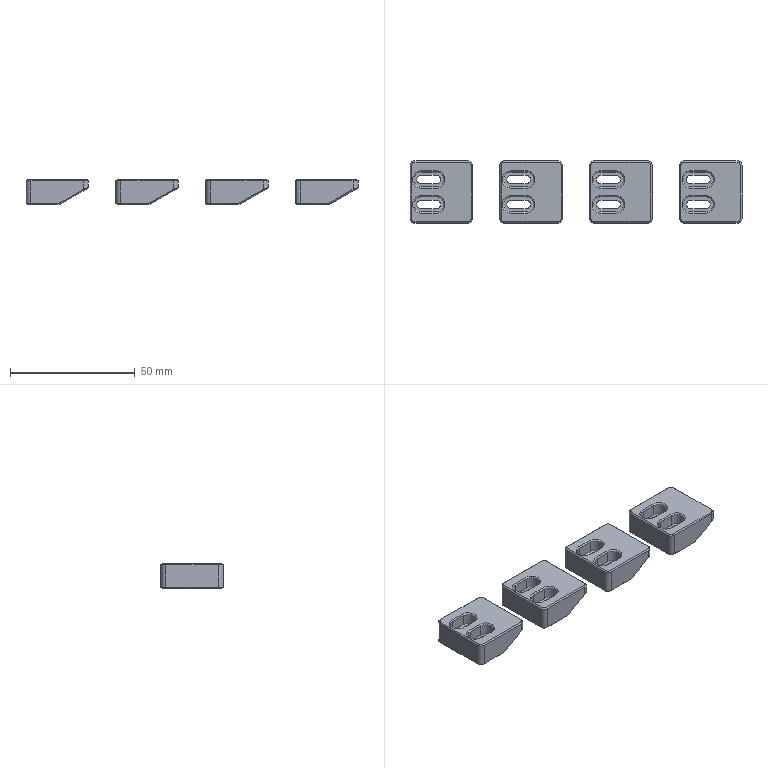NC program | NX | posted with a generic post | part box 133 x 25 x 10 mm
Lines 51 to 970 of 3677:
(ZLEVEL_PROFILE_COPY_COPY , TOOL : D4)
N100 T11 M6
N102 G54
N104 G17 G0 G90 X59.704 Y-4. S9500 M3
N106 G43 Z30. H11
N108 Z1.5
N110 G94 G1 X55.905 Z1.301 F1350.
N112 X55.631 Y-4.061 Z1.286
N114 X55.457 Y-4.158 Z1.276
N116 X55.261 Y-4.358 Z1.261
N118 X55.11 Y-4.603 Z1.246
N120 X55.004 Y-4.807 Z1.234
N122 X55.003 Y-5.188 Z1.214
N124 X55.113 Y-5.404 Z1.201
N126 X55.192 Y-5.615 Z1.19
N128 X55.32 Y-5.757 Z1.179
N130 X55.53 Y-5.86 Z1.167
N132 X55.597 Y-5.888 Z1.163
N134 X55.987 Y-5.982 Z1.142
N136 Y-6. Z1.141
N138 X62.118 Z0.82
N140 X62.329 Y-5.926 Z0.808
N142 X62.561 Y-5.847 Z0.796
N144 X62.879 Y-5.518 Z0.772
N146 X63.02 Y-5.083 Z0.748
N148 X62.944 Y-4.599 Z0.722
N150 X62.674 Y-4.229 Z0.698
N152 X62.269 Y-4.015 Z0.674
N154 X62.025 Y-4.012 Z0.661
N156 Y-4.
N158 X55.905 Z0.34
N160 X55.631 Y-4.061 Z0.325
N162 X55.457 Y-4.158 Z0.315
N164 X55.261 Y-4.358 Z0.3
N166 X55.11 Y-4.603 Z0.285
N168 X55.004 Y-4.807 Z0.273
N170 X55.003 Y-5.188 Z0.253
N172 X55.113 Y-5.404 Z0.24
N174 X55.192 Y-5.615 Z0.228
N176 X55.32 Y-5.757 Z0.218
N178 X55.53 Y-5.86 Z0.206
N180 X55.597 Y-5.888 Z0.202
N182 X55.987 Y-5.982 Z0.181
N184 Y-6. Z0.18
N186 X62.118 Z-0.141
N188 X62.329 Y-5.926 Z-0.153
N190 X62.561 Y-5.847 Z-0.166
N192 X62.879 Y-5.518 Z-0.19
N194 X63.02 Y-5.083 Z-0.214
N196 X62.944 Y-4.599 Z-0.239
N198 X62.674 Y-4.229 Z-0.263
N200 X62.269 Y-4.015 Z-0.287
N202 X62.025 Y-4.012 Z-0.3
N204 Y-4.
N206 X55.905
N208 G3 X55.261 Y-4.358 R1.295
N210 G1 X55.11 Y-4.603
N212 G3 X55.113 Y-5.404 R0.863
N214 X55.53 Y-5.86 R0.828
N216 G1 X55.597 Y-5.888
N218 X55.987 Y-5.982
N220 Y-6.
N222 X62.118
N224 X62.329 Y-5.926
N226 G3 X62.025 Y-4.012 R0.984
N228 G1 X61.786 Y-4. Z-0.305
N230 X61.548 Z-0.311
N232 X56.176 Z-0.429
N234 X55.822 Y-4.041 Z-0.436
N236 X55.7 Y-4.069 Z-0.439
N238 X55.438 Y-4.201 Z-0.446
N240 X55.288 Y-4.326 Z-0.45
N242 X55.128 Y-4.561 Z-0.456
N244 X55.049 Y-4.75 Z-0.461
N246 X55.027 Y-4.927 Z-0.465
N248 X55.019 Y-5.016 Z-0.467
N250 X55.029 Y-5.087 Z-0.468
N252 X55.048 Y-5.231 Z-0.471
N254 X55.114 Y-5.41 Z-0.476
N256 X55.152 Y-5.497 Z-0.478
N258 X55.275 Y-5.656 Z-0.482
N260 X55.407 Y-5.775 Z-0.486
N262 X55.478 Y-5.828 Z-0.488
N264 X55.541 Y-5.864 Z-0.49
N266 X55.677 Y-5.92 Z-0.493
N268 X55.877 Y-5.967 Z-0.498
N270 X56.141 Y-6. Z-0.504
N272 X60.536 Z-0.6
N274 X62.
N276 G3 X62.025 Y-4. R1.
N278 G1 X61.78 Z-0.605
N280 X59.576 Z-0.654
N282 X57.617 Z-0.696
N284 X57.372 Y-4.001 Z-0.702
N286 X57.128 Y-4. Z-0.707
N288 X56.148 Z-0.729
N290 X55.807 Y-4.043 Z-0.736
N292 X55.673 Y-4.08 Z-0.739
N294 X55.42 Y-4.218 Z-0.746
N296 X55.277 Y-4.34 Z-0.75
N298 X55.123 Y-4.571 Z-0.756
N300 X55.048 Y-4.757 Z-0.761
N302 X55.02 Y-5.023 Z-0.767
N304 X55.048 Y-5.233 Z-0.771
N306 X55.112 Y-5.406 Z-0.776
N308 X55.149 Y-5.491 Z-0.778
N310 X55.271 Y-5.652 Z-0.782
N312 X55.404 Y-5.771 Z-0.786
N314 X55.474 Y-5.826 Z-0.788
N316 X55.533 Y-5.862 Z-0.79
N318 X55.664 Y-5.917 Z-0.793
N320 X55.868 Y-5.965 Z-0.798
N322 X56.138 Y-6. Z-0.804
N324 X60.546 Z-0.9
N326 X62.
N328 G3 X62.025 Y-4. R1.
N330 G1 X61.78 Z-0.905
N332 X59.576 Z-0.954
N334 X56.638 Z-1.018
N336 X56.393 Y-4.001 Z-1.023
N338 X56.148 Y-4. Z-1.029
N340 X55.809 Y-4.043 Z-1.036
N342 X55.673 Y-4.08 Z-1.039
N344 X55.421 Y-4.217 Z-1.046
N346 X55.277 Y-4.341 Z-1.05
N348 X55.123 Y-4.571 Z-1.056
N350 X55.048 Y-4.757 Z-1.061
N352 X55.021 Y-5.023 Z-1.067
N354 X55.048 Y-5.233 Z-1.071
N356 X55.113 Y-5.406 Z-1.076
N358 X55.149 Y-5.49 Z-1.078
N360 X55.271 Y-5.652 Z-1.082
N362 X55.404 Y-5.771 Z-1.086
N364 X55.474 Y-5.825 Z-1.088
N366 X55.533 Y-5.862 Z-1.09
N368 X55.664 Y-5.917 Z-1.093
N370 X55.868 Y-5.965 Z-1.098
N372 X56.138 Y-6. Z-1.104
N374 X60.546 Z-1.2
N376 X62.
N378 G3 X62.025 Y-4. R1.
N380 G1 X61.78 Z-1.205
N382 X59.576 Z-1.254
N384 X56.148 Z-1.329
N386 X55.807 Y-4.043 Z-1.336
N388 X55.673 Y-4.08 Z-1.339
N390 X55.419 Y-4.216 Z-1.346
N392 X55.277 Y-4.341 Z-1.35
N394 X55.121 Y-4.575 Z-1.356
N396 X55.048 Y-4.757 Z-1.361
N398 X55.021 Y-5.024 Z-1.367
N400 X55.048 Y-5.233 Z-1.371
N402 X55.113 Y-5.406 Z-1.376
N404 X55.15 Y-5.49 Z-1.378
N406 X55.271 Y-5.652 Z-1.382
N408 X55.404 Y-5.77 Z-1.386
N410 X55.474 Y-5.825 Z-1.388
N412 X55.533 Y-5.862 Z-1.39
N414 X55.664 Y-5.917 Z-1.393
N416 X55.868 Y-5.965 Z-1.398
N418 X56.138 Y-6. Z-1.404
N420 X60.546 Z-1.5
N422 X62.
N424 G3 X62.025 Y-4. R1.
N426 G1 X61.78 Z-1.505
N428 X59.576 Z-1.554
N430 X56.148 Z-1.629
N432 X55.807 Y-4.043 Z-1.636
N434 X55.673 Y-4.08 Z-1.639
N436 X55.42 Y-4.216 Z-1.646
N438 X55.277 Y-4.341 Z-1.65
N440 X55.122 Y-4.575 Z-1.656
N442 X55.048 Y-4.757 Z-1.661
N444 X55.021 Y-5.023 Z-1.667
N446 X55.048 Y-5.233 Z-1.671
N448 X55.113 Y-5.406 Z-1.676
N450 X55.15 Y-5.49 Z-1.678
N452 X55.271 Y-5.652 Z-1.682
N454 X55.404 Y-5.77 Z-1.686
N456 X55.473 Y-5.824 Z-1.688
N458 X55.533 Y-5.861 Z-1.69
N460 X55.664 Y-5.917 Z-1.693
N462 X55.867 Y-5.964 Z-1.698
N464 X56.138 Y-6. Z-1.704
N466 X60.546 Z-1.8
N468 X62.
N470 G3 X62.025 Y-4. R1.
N472 G1 X61.78 Z-1.805
N474 X59.576 Z-1.854
N476 X57.128 Z-1.907
N478 X56.883 Y-4.001 Z-1.913
N480 X56.638 Y-4. Z-1.918
N482 X56.148 Z-1.929
N484 X55.808 Y-4.044 Z-1.936
N486 X55.673 Y-4.08 Z-1.939
N488 X55.42 Y-4.216 Z-1.946
N490 X55.277 Y-4.341 Z-1.95
N492 X55.122 Y-4.575 Z-1.956
N494 X55.048 Y-4.757 Z-1.961
N496 X55.021 Y-5.023 Z-1.967
N498 X55.049 Y-5.233 Z-1.971
N500 X55.114 Y-5.405 Z-1.976
N502 X55.148 Y-5.491 Z-1.978
N504 X55.271 Y-5.652 Z-1.982
N506 X55.405 Y-5.771 Z-1.986
N508 X55.475 Y-5.825 Z-1.988
N510 X55.535 Y-5.862 Z-1.99
N512 X55.664 Y-5.917 Z-1.993
N514 X55.868 Y-5.964 Z-1.998
N516 X56.138 Y-6. Z-2.004
N518 X60.546 Z-2.1
N520 X62.
N522 G3 X62.025 Y-4. R1.
N524 G1 X61.78 Z-2.105
N526 X59.576 Z-2.154
N528 X56.148 Z-2.229
N530 X55.808 Y-4.044 Z-2.236
N532 X55.673 Y-4.08 Z-2.239
N534 X55.42 Y-4.216 Z-2.246
N536 X55.277 Y-4.341 Z-2.25
N538 X55.123 Y-4.575 Z-2.256
N540 X55.049 Y-4.757 Z-2.261
N542 X55.022 Y-5.023 Z-2.267
N544 X55.049 Y-5.233 Z-2.271
N546 X55.114 Y-5.405 Z-2.276
N548 X55.148 Y-5.49 Z-2.278
N550 X55.271 Y-5.652 Z-2.282
N552 X55.405 Y-5.77 Z-2.286
N554 X55.475 Y-5.825 Z-2.288
N556 X55.534 Y-5.862 Z-2.29
N558 X55.664 Y-5.917 Z-2.293
N560 X55.868 Y-5.964 Z-2.298
N562 X56.138 Y-6. Z-2.304
N564 X60.546 Z-2.4
N566 X62.
N568 G3 X62.025 Y-4. R1.
N570 G1 X61.78 Z-2.405
N572 X59.576 Z-2.454
N574 X56.148 Z-2.529
N576 X55.808 Y-4.044 Z-2.536
N578 X55.673 Y-4.08 Z-2.539
N580 X55.421 Y-4.216 Z-2.546
N582 X55.277 Y-4.341 Z-2.55
N584 X55.123 Y-4.574 Z-2.556
N586 X55.049 Y-4.757 Z-2.561
N588 X55.028 Y-4.934 Z-2.565
N590 X55.019 Y-5.022 Z-2.567
N592 X55.029 Y-5.092 Z-2.568
N594 X55.049 Y-5.233 Z-2.571
N596 X55.115 Y-5.407 Z-2.576
N598 X55.152 Y-5.493 Z-2.578
N600 X55.271 Y-5.652 Z-2.582
N602 X55.404 Y-5.769 Z-2.586
N604 X55.474 Y-5.824 Z-2.588
N606 X55.533 Y-5.861 Z-2.59
N608 X55.664 Y-5.916 Z-2.593
N610 X55.867 Y-5.964 Z-2.597
N612 X56.138 Y-6. Z-2.604
N614 X60.546 Z-2.7
N616 X62.
N618 G3 X62.025 Y-4. R1.
N620 G1 X61.78 Z-2.705
N622 X59.576 Z-2.754
N624 X56.148 Z-2.829
N626 X55.808 Y-4.044 Z-2.836
N628 X55.673 Y-4.08 Z-2.839
N630 X55.421 Y-4.216 Z-2.846
N632 X55.278 Y-4.341 Z-2.85
N634 X55.123 Y-4.574 Z-2.856
N636 X55.049 Y-4.757 Z-2.861
N638 X55.02 Y-5.022 Z-2.867
N640 X55.049 Y-5.233 Z-2.871
N642 X55.115 Y-5.407 Z-2.876
N644 X55.15 Y-5.493 Z-2.878
N646 X55.271 Y-5.652 Z-2.882
N648 X55.476 Y-5.824 Z-2.888
N650 X55.664 Y-5.916 Z-2.893
N652 X55.844 Y-5.962 Z-2.897
N654 X56.138 Y-6. Z-2.904
N656 X60.546 Z-3.
N658 X62.
N660 G3 X62.025 Y-4. R1.
N662 G1 X61.78 Z-3.005
N664 X59.576 Z-3.054
N666 X56.148 Z-3.129
N668 X55.809 Y-4.044 Z-3.136
N670 X55.673 Y-4.081 Z-3.139
N672 X55.422 Y-4.217 Z-3.146
N674 X55.278 Y-4.341 Z-3.15
N676 X55.124 Y-4.573 Z-3.156
N678 X55.049 Y-4.757 Z-3.161
N680 X55.02 Y-5.022 Z-3.167
N682 X55.049 Y-5.233 Z-3.171
N684 X55.115 Y-5.407 Z-3.176
N686 X55.15 Y-5.493 Z-3.178
N688 X55.271 Y-5.652 Z-3.182
N690 X55.476 Y-5.824 Z-3.188
N692 X55.664 Y-5.916 Z-3.193
N694 X55.844 Y-5.961 Z-3.197
N696 X56.138 Y-6. Z-3.204
N698 X60.546 Z-3.3
N700 X62.
N702 G3 X62.025 Y-4. R1.
N704 G1 X61.78 Z-3.305
N706 X59.576 Z-3.354
N708 X56.148 Z-3.429
N710 X55.808 Y-4.043 Z-3.436
N712 X55.673 Y-4.081 Z-3.439
N714 X55.418 Y-4.219 Z-3.446
N716 X55.278 Y-4.341 Z-3.45
N718 X55.123 Y-4.575 Z-3.456
N720 X55.049 Y-4.757 Z-3.461
N722 X55.02 Y-5.022 Z-3.467
N724 X55.049 Y-5.233 Z-3.471
N726 X55.116 Y-5.406 Z-3.476
N728 X55.15 Y-5.493 Z-3.478
N730 X55.271 Y-5.652 Z-3.482
N732 X55.476 Y-5.824 Z-3.488
N734 X55.664 Y-5.916 Z-3.493
N736 X55.844 Y-5.961 Z-3.497
N738 X56.138 Y-6. Z-3.504
N740 X60.546 Z-3.6
N742 X62.
N744 G3 X62.025 Y-4. R1.
N746 G1 X61.78 Z-3.605
N748 X59.576 Z-3.654
N750 X57.617 Z-3.696
N752 X57.372 Y-4.002 Z-3.702
N754 X57.128 Y-4. Z-3.707
N756 X56.148 Z-3.729
N758 X55.809 Y-4.043 Z-3.736
N760 X55.673 Y-4.081 Z-3.739
N762 X55.418 Y-4.219 Z-3.746
N764 X55.278 Y-4.341 Z-3.75
N766 X55.122 Y-4.573 Z-3.756
N768 X55.049 Y-4.757 Z-3.761
N770 X55.02 Y-5.025 Z-3.767
N772 X55.049 Y-5.233 Z-3.771
N774 X55.116 Y-5.407 Z-3.776
N776 X55.15 Y-5.493 Z-3.778
N778 X55.271 Y-5.652 Z-3.782
N780 X55.404 Y-5.771 Z-3.786
N782 X55.475 Y-5.826 Z-3.788
N784 X55.535 Y-5.86 Z-3.79
N786 X55.664 Y-5.916 Z-3.793
N788 X55.867 Y-5.965 Z-3.798
N790 X56.138 Y-6. Z-3.804
N792 X60.546 Z-3.9
N794 X62.
N796 G3 X62.025 Y-4. R1.
N798 G1 X61.78 Z-3.905
N800 X56.148 Z-4.018
N802 X55.809 Y-4.043 Z-4.025
N804 X55.673 Y-4.081 Z-4.028
N806 X55.419 Y-4.219 Z-4.034
N808 X55.278 Y-4.341 Z-4.038
N810 X55.122 Y-4.573 Z-4.043
N812 X55.049 Y-4.757 Z-4.047
N814 X55.02 Y-5.025 Z-4.053
N816 X55.049 Y-5.233 Z-4.057
N818 X55.116 Y-5.406 Z-4.061
N820 X55.15 Y-5.493 Z-4.063
N822 X55.271 Y-5.652 Z-4.067
N824 X55.404 Y-5.771 Z-4.071
N826 X55.475 Y-5.825 Z-4.072
N828 X55.535 Y-5.86 Z-4.074
N830 X55.664 Y-5.916 Z-4.077
N832 X55.867 Y-5.965 Z-4.081
N834 X56.138 Y-6. Z-4.087
N836 X60.546 Z-4.175
N838 X62.
N840 G3 X62.025 Y-4. R1.
N842 G1 X61.78 Z-4.18
N844 X57.617 Z-4.263
N846 X57.372 Y-4.002 Z-4.268
N848 X57.128 Y-4. Z-4.273
N850 X56.148 Z-4.293
N852 X55.809 Y-4.043 Z-4.3
N854 X55.673 Y-4.081 Z-4.303
N856 X55.419 Y-4.219 Z-4.309
N858 X55.278 Y-4.341 Z-4.313
N860 X55.122 Y-4.573 Z-4.318
N862 X55.049 Y-4.758 Z-4.322
N864 X55.021 Y-5.025 Z-4.328
N866 X55.049 Y-5.233 Z-4.332
N868 X55.114 Y-5.408 Z-4.336
N870 X55.15 Y-5.493 Z-4.338
N872 X55.272 Y-5.652 Z-4.342
N874 X55.404 Y-5.771 Z-4.346
N876 X55.474 Y-5.825 Z-4.347
N878 X55.535 Y-5.86 Z-4.349
N880 X55.664 Y-5.916 Z-4.352
N882 X55.867 Y-5.965 Z-4.356
N884 X56.138 Y-6. Z-4.362
N886 X60.546 Z-4.45
N888 X62.
N890 G3 X62.025 Y-4. R1.
N892 G1 X61.78 Z-4.455
N894 X56.148 Z-4.568
N896 X55.809 Y-4.043 Z-4.575
N898 X55.673 Y-4.081 Z-4.578
N900 X55.419 Y-4.219 Z-4.584
N902 X55.278 Y-4.341 Z-4.588
N904 X55.123 Y-4.573 Z-4.593
N906 X55.049 Y-4.758 Z-4.597
N908 X55.021 Y-5.025 Z-4.603
N910 X55.05 Y-5.233 Z-4.607
N912 X55.114 Y-5.407 Z-4.611
N914 X55.151 Y-5.492 Z-4.613
N916 X55.272 Y-5.651 Z-4.617
N918 X55.404 Y-5.77 Z-4.621
N920 X55.473 Y-5.824 Z-4.622
N922 X55.534 Y-5.859 Z-4.624
N924 X55.664 Y-5.916 Z-4.627
N926 X55.866 Y-5.964 Z-4.631
N928 X56.138 Y-6. Z-4.637
N930 X60.546 Z-4.725
N932 X62.
N934 G3 X62.025 Y-4. R1.
N936 G1 X61.78 Z-4.73
N938 X56.148 Z-4.843
N940 X55.809 Y-4.043 Z-4.85
N942 X55.673 Y-4.081 Z-4.853
N944 X55.42 Y-4.219 Z-4.859
N946 X55.278 Y-4.342 Z-4.863
N948 X55.123 Y-4.572 Z-4.868
N950 X55.05 Y-4.758 Z-4.872
N952 X55.022 Y-5.025 Z-4.878
N954 X55.05 Y-5.233 Z-4.882
N956 X55.114 Y-5.406 Z-4.886
N958 X55.151 Y-5.491 Z-4.888
N960 X55.272 Y-5.651 Z-4.892
N962 X55.403 Y-5.77 Z-4.896
N964 X55.473 Y-5.823 Z-4.897
N966 X55.534 Y-5.859 Z-4.899
N968 X55.664 Y-5.916 Z-4.902
N970 X55.866 Y-5.964 Z-4.906
N972 X56.138 Y-6. Z-4.912
N974 X60.546 Z-5.
N976 X62.
N978 G3 X63. Y-5. R1.
N980 X62. Y-4. R1.
N982 G1 X55.986
N984 G3 X56. Y-6. R1.
N986 G1 X60.546
N988 Z-3.5
N990 G0 Z30.
N992 X59.685 Y6.
N994 Z1.5
N996 G1 X55.844 Z1.299
N998 X55.522 Y5.856 Z1.28
N1000 X55.32 Y5.757 Z1.268
N1002 X55.192 Y5.615 Z1.258
N1004 X55.108 Y5.392 Z1.246
N1006 X55.003 Y5.188 Z1.234
N1008 X55.004 Y4.807 Z1.214
N1010 X55.11 Y4.603 Z1.202
N1012 X55.247 Y4.382 Z1.188
N1014 X55.404 Y4.191 Z1.175
N1016 X55.74 Y4.026 Z1.156
N1018 X55.987 Y4.019 Z1.143
N1020 Y4. Z1.142
N1022 X62.139 Z0.819
N1024 X62.398 Y4.101 Z0.805
N1026 X62.623 Y4.199 Z0.792
N1028 X62.906 Y4.533 Z0.769
N1030 X63.021 Y4.956 Z0.746
N1032 X62.926 Y5.436 Z0.72
N1034 X62.658 Y5.783 Z0.697
N1036 X62.27 Y5.985 Z0.674
N1038 X62.025 Y5.989 Z0.662
N1040 Y6. Z0.661
N1042 X55.844 Z0.337
N1044 X55.522 Y5.856 Z0.319
N1046 X55.32 Y5.757 Z0.307
N1048 X55.192 Y5.615 Z0.297
N1050 X55.108 Y5.392 Z0.284
N1052 X55.003 Y5.188 Z0.272
N1054 X55.004 Y4.807 Z0.252
N1056 X55.11 Y4.603 Z0.24
N1058 X55.247 Y4.382 Z0.227
N1060 X55.404 Y4.191 Z0.214
N1062 X55.74 Y4.026 Z0.194
N1064 X55.987 Y4.019 Z0.181
N1066 Y4. Z0.18
N1068 X62.139 Z-0.142
N1070 X62.398 Y4.101 Z-0.157
N1072 X62.623 Y4.199 Z-0.17
N1074 X62.906 Y4.533 Z-0.193
N1076 X63.021 Y4.956 Z-0.216
N1078 X62.926 Y5.436 Z-0.241
N1080 X62.658 Y5.783 Z-0.264
N1082 X62.27 Y5.985 Z-0.287
N1084 X62.025 Y5.989 Z-0.3
N1086 Y6.
N1088 X55.844
N1090 X55.522 Y5.856
N1092 G3 X55.108 Y5.392 R0.829
N1094 X55.11 Y4.603 R0.862
N1096 G1 X55.247 Y4.382
N1098 G3 X55.987 Y4.019 R1.002
N1100 G1 Y4.
N1102 X62.139
N1104 X62.398 Y4.101
N1106 G3 X62.025 Y5.989 R0.984
N1108 G1 X61.786 Y6. Z-0.305
N1110 X61.547 Z-0.311
N1112 X56.174 Z-0.429
N1114 X55.823 Y5.96 Z-0.436
N1116 X55.701 Y5.931 Z-0.439
N1118 X55.442 Y5.801 Z-0.446
N1120 X55.292 Y5.677 Z-0.45
N1122 X55.129 Y5.446 Z-0.456
N1124 X55.052 Y5.258 Z-0.461
N1126 X55.028 Y5.076 Z-0.465
N1128 X55.019 Y4.985 Z-0.467
N1130 X55.027 Y4.916 Z-0.468
N1132 X55.046 Y4.777 Z-0.471
N1134 X55.111 Y4.597 Z-0.476
N1136 X55.148 Y4.509 Z-0.478
N1138 X55.271 Y4.348 Z-0.482
N1140 X55.408 Y4.226 Z-0.486
N1142 X55.479 Y4.17 Z-0.488
N1144 X55.541 Y4.135 Z-0.49
N1146 X55.674 Y4.079 Z-0.493
N1148 X55.869 Y4.035 Z-0.497
N1150 X56.137 Y4. Z-0.504
N1152 X60.533 Z-0.6
N1154 X62.
N1156 G3 X62.025 Y6. R1.
N1158 G1 X61.78 Z-0.605
N1160 X59.821 Z-0.648
N1162 X57.617 Z-0.696
N1164 X57.373 Y5.999 Z-0.702
N1166 X57.128 Y6. Z-0.707
N1168 X56.638 Z-0.718
N1170 X56.393 Y5.999 Z-0.723
N1172 X56.148 Y6. Z-0.729
N1174 X55.809 Y5.957 Z-0.736
N1176 X55.673 Y5.92 Z-0.739
N1178 X55.421 Y5.783 Z-0.746
N1180 X55.277 Y5.66 Z-0.75
N1182 X55.123 Y5.429 Z-0.756
N1184 X55.048 Y5.243 Z-0.761
N1186 X55.02 Y4.977 Z-0.767
N1188 X55.048 Y4.767 Z-0.771
N1190 X55.112 Y4.594 Z-0.776
N1192 X55.149 Y4.51 Z-0.778
N1194 X55.271 Y4.348 Z-0.782
N1196 X55.404 Y4.229 Z-0.786
N1198 X55.474 Y4.174 Z-0.788
N1200 X55.533 Y4.138 Z-0.79
N1202 X55.664 Y4.083 Z-0.793
N1204 X55.868 Y4.035 Z-0.798
N1206 X56.138 Y4. Z-0.804
N1208 X60.546 Z-0.9
N1210 X62.
N1212 G3 X62.025 Y6. R1.
N1214 G1 X61.78 Z-0.905
N1216 X59.821 Z-0.948
N1218 X56.148 Z-1.029
N1220 X55.807 Y5.957 Z-1.036
N1222 X55.673 Y5.92 Z-1.039
N1224 X55.421 Y5.782 Z-1.046
N1226 X55.277 Y5.659 Z-1.05
N1228 X55.123 Y5.429 Z-1.056
N1230 X55.048 Y5.243 Z-1.061
N1232 X55.021 Y4.977 Z-1.067
N1234 X55.048 Y4.767 Z-1.071
N1236 X55.113 Y4.594 Z-1.076
N1238 X55.149 Y4.51 Z-1.078
N1240 X55.271 Y4.348 Z-1.082
N1242 X55.404 Y4.229 Z-1.086
N1244 X55.474 Y4.175 Z-1.088
N1246 X55.533 Y4.138 Z-1.09
N1248 X55.664 Y4.083 Z-1.093
N1250 X55.868 Y4.035 Z-1.098
N1252 X56.138 Y4. Z-1.104
N1254 X60.546 Z-1.2
N1256 X62.
N1258 G3 X62.025 Y6. R1.
N1260 G1 X61.78 Z-1.205
N1262 X59.821 Z-1.248
N1264 X56.148 Z-1.329
N1266 X55.807 Y5.957 Z-1.336
N1268 X55.673 Y5.92 Z-1.339
N1270 X55.419 Y5.784 Z-1.346
N1272 X55.277 Y5.659 Z-1.35
N1274 X55.121 Y5.425 Z-1.356
N1276 X55.048 Y5.243 Z-1.361
N1278 X55.021 Y4.976 Z-1.367
N1280 X55.048 Y4.767 Z-1.371
N1282 X55.113 Y4.594 Z-1.376
N1284 X55.15 Y4.51 Z-1.378
N1286 X55.271 Y4.348 Z-1.382
N1288 X55.404 Y4.23 Z-1.386
N1290 X55.474 Y4.175 Z-1.388
N1292 X55.533 Y4.138 Z-1.39
N1294 X55.664 Y4.083 Z-1.393
N1296 X55.868 Y4.035 Z-1.398
N1298 X56.138 Y4. Z-1.404
N1300 X60.546 Z-1.5
N1302 X62.
N1304 G3 X62.025 Y6. R1.
N1306 G1 X61.78 Z-1.505
N1308 X59.821 Z-1.548
N1310 X56.148 Z-1.629
N1312 X55.807 Y5.957 Z-1.636
N1314 X55.673 Y5.92 Z-1.639
N1316 X55.42 Y5.784 Z-1.646
N1318 X55.277 Y5.659 Z-1.65
N1320 X55.122 Y5.425 Z-1.656
N1322 X55.048 Y5.243 Z-1.661
N1324 X55.021 Y4.977 Z-1.667
N1326 X55.048 Y4.767 Z-1.671
N1328 X55.113 Y4.594 Z-1.676
N1330 X55.15 Y4.51 Z-1.678
N1332 X55.271 Y4.348 Z-1.682
N1334 X55.404 Y4.23 Z-1.686
N1336 X55.473 Y4.176 Z-1.688
N1338 X55.533 Y4.139 Z-1.69
N1340 X55.664 Y4.083 Z-1.693
N1342 X55.867 Y4.036 Z-1.698
N1344 X56.138 Y4. Z-1.704
N1346 X60.546 Z-1.8
N1348 X62.
N1350 G3 X62.025 Y6. R1.
N1352 G1 X61.78 Z-1.805
N1354 X59.821 Z-1.848
N1356 X56.148 Z-1.929
N1358 X55.808 Y5.956 Z-1.936
N1360 X55.673 Y5.92 Z-1.939
N1362 X55.42 Y5.784 Z-1.946
N1364 X55.277 Y5.659 Z-1.95
N1366 X55.122 Y5.425 Z-1.956
N1368 X55.048 Y5.243 Z-1.961
N1370 X55.021 Y4.977 Z-1.967
N1372 X55.049 Y4.767 Z-1.971
N1374 X55.114 Y4.595 Z-1.976
N1376 X55.147 Y4.509 Z-1.978
N1378 X55.271 Y4.348 Z-1.982
N1380 X55.405 Y4.229 Z-1.986
N1382 X55.475 Y4.175 Z-1.988
N1384 X55.534 Y4.138 Z-1.99
N1386 X55.664 Y4.083 Z-1.993
N1388 X55.868 Y4.036 Z-1.998
N1390 X56.138 Y4. Z-2.004
N1392 X60.546 Z-2.1
N1394 X62.
N1396 G3 X62.025 Y6. R1.
N1398 G1 X61.78 Z-2.105
N1400 X59.821 Z-2.148
N1402 X56.148 Z-2.229
N1404 X55.808 Y5.956 Z-2.236
N1406 X55.673 Y5.92 Z-2.239
N1408 X55.42 Y5.784 Z-2.246
N1410 X55.277 Y5.659 Z-2.25
N1412 X55.123 Y5.426 Z-2.256
N1414 X55.049 Y5.243 Z-2.261
N1416 X55.022 Y4.978 Z-2.267
N1418 X55.049 Y4.767 Z-2.271
N1420 X55.114 Y4.595 Z-2.276
N1422 X55.148 Y4.51 Z-2.278
N1424 X55.271 Y4.348 Z-2.282
N1426 X55.405 Y4.23 Z-2.286
N1428 X55.475 Y4.175 Z-2.288
N1430 X55.534 Y4.139 Z-2.29
N1432 X55.664 Y4.084 Z-2.293
N1434 X55.868 Y4.036 Z-2.298
N1436 X56.138 Y4. Z-2.304
N1438 X60.546 Z-2.4
N1440 X62.
N1442 G3 X62.025 Y6. R1.
N1444 G1 X61.78 Z-2.405
N1446 X59.821 Z-2.448
N1448 X56.148 Z-2.529
N1450 X55.808 Y5.956 Z-2.536
N1452 X55.673 Y5.92 Z-2.539
N1454 X55.421 Y5.784 Z-2.546
N1456 X55.278 Y5.659 Z-2.55
N1458 X55.123 Y5.426 Z-2.556
N1460 X55.049 Y5.243 Z-2.561
N1462 X55.028 Y5.066 Z-2.565
N1464 X55.019 Y4.978 Z-2.567
N1466 X55.029 Y4.908 Z-2.568
N1468 X55.049 Y4.767 Z-2.571
N1470 X55.115 Y4.593 Z-2.576
N1472 X55.152 Y4.507 Z-2.578
N1474 X55.271 Y4.348 Z-2.582
N1476 X55.404 Y4.231 Z-2.586
N1478 X55.474 Y4.176 Z-2.588
N1480 X55.533 Y4.139 Z-2.59
N1482 X55.664 Y4.084 Z-2.593
N1484 X55.867 Y4.036 Z-2.597
N1486 X56.138 Y4. Z-2.604
N1488 X60.546 Z-2.7
N1490 X62.
N1492 G3 X62.025 Y6. R1.
N1494 G1 X61.78 Z-2.705
N1496 X59.821 Z-2.748
N1498 X56.148 Z-2.829
N1500 X55.808 Y5.956 Z-2.836
N1502 X55.673 Y5.92 Z-2.839
N1504 X55.421 Y5.784 Z-2.846
N1506 X55.278 Y5.659 Z-2.85
N1508 X55.123 Y5.426 Z-2.856
N1510 X55.049 Y5.243 Z-2.861
N1512 X55.02 Y4.978 Z-2.867
N1514 X55.049 Y4.767 Z-2.871
N1516 X55.115 Y4.593 Z-2.876
N1518 X55.15 Y4.507 Z-2.878
N1520 X55.271 Y4.348 Z-2.882
N1522 X55.476 Y4.176 Z-2.888
N1524 X55.664 Y4.084 Z-2.893
N1526 X55.844 Y4.038 Z-2.897
N1528 X56.138 Y4. Z-2.904
N1530 X60.546 Z-3.
N1532 X62.
N1534 G3 X62.025 Y6. R1.
N1536 G1 X61.78 Z-3.005
N1538 X59.821 Z-3.048
N1540 X56.148 Z-3.129
N1542 X55.809 Y5.956 Z-3.136
N1544 X55.673 Y5.919 Z-3.139
N1546 X55.422 Y5.783 Z-3.146
N1548 X55.278 Y5.659 Z-3.15
N1550 X55.124 Y5.427 Z-3.156
N1552 X55.049 Y5.243 Z-3.161
N1554 X55.02 Y4.978 Z-3.167
N1556 X55.049 Y4.767 Z-3.171
N1558 X55.115 Y4.594 Z-3.176
N1560 X55.15 Y4.507 Z-3.178
N1562 X55.271 Y4.348 Z-3.182
N1564 X55.476 Y4.176 Z-3.188
N1566 X55.664 Y4.084 Z-3.193
N1568 X55.844 Y4.039 Z-3.197
N1570 X56.138 Y4. Z-3.204
N1572 X60.546 Z-3.3
N1574 X62.
N1576 G3 X62.025 Y6. R1.
N1578 G1 X61.78 Z-3.305
N1580 X59.821 Z-3.348
N1582 X56.148 Z-3.429
N1584 X55.808 Y5.957 Z-3.436
N1586 X55.673 Y5.919 Z-3.439
N1588 X55.418 Y5.781 Z-3.446
N1590 X55.278 Y5.659 Z-3.45
N1592 X55.123 Y5.425 Z-3.456
N1594 X55.049 Y5.243 Z-3.461
N1596 X55.02 Y4.978 Z-3.467
N1598 X55.049 Y4.767 Z-3.471
N1600 X55.115 Y4.594 Z-3.476
N1602 X55.15 Y4.507 Z-3.478
N1604 X55.271 Y4.348 Z-3.482
N1606 X55.476 Y4.176 Z-3.488
N1608 X55.664 Y4.084 Z-3.493
N1610 X55.844 Y4.039 Z-3.497
N1612 X56.138 Y4. Z-3.504
N1614 X60.546 Z-3.6
N1616 X62.
N1618 G3 X62.025 Y6. R1.
N1620 G1 X61.78 Z-3.605
N1622 X59.821 Z-3.648
N1624 X57.617 Z-3.696
N1626 X57.373 Y5.998 Z-3.702
N1628 X57.128 Y6. Z-3.707
N1630 X56.883 Y5.998 Z-3.713
N1632 X56.638 Y6. Z-3.718
N1634 X56.148 Z-3.729
N1636 X55.809 Y5.957 Z-3.736
N1638 X55.673 Y5.919 Z-3.739
N1640 X55.418 Y5.781 Z-3.746
N1642 X55.278 Y5.659 Z-3.75
N1644 X55.122 Y5.427 Z-3.756
N1646 X55.049 Y5.243 Z-3.761
N1648 X55.02 Y4.975 Z-3.767
N1650 X55.049 Y4.767 Z-3.771
N1652 X55.116 Y4.594 Z-3.776
N1654 X55.15 Y4.507 Z-3.778
N1656 X55.271 Y4.348 Z-3.782
N1658 X55.476 Y4.177 Z-3.788
N1660 X55.664 Y4.084 Z-3.793
N1662 X55.844 Y4.039 Z-3.797
N1664 X56.138 Y4. Z-3.804
N1666 X60.546 Z-3.9
N1668 X62.
N1670 G3 X62.025 Y6. R1.
N1672 G1 X61.78 Z-3.905
N1674 X56.148 Z-4.018
N1676 X55.809 Y5.957 Z-4.025
N1678 X55.673 Y5.919 Z-4.028
N1680 X55.419 Y5.781 Z-4.034
N1682 X55.278 Y5.659 Z-4.038
N1684 X55.122 Y5.427 Z-4.043
N1686 X55.049 Y5.243 Z-4.047
N1688 X55.02 Y4.975 Z-4.053
N1690 X55.049 Y4.767 Z-4.057
N1692 X55.116 Y4.594 Z-4.061
N1694 X55.15 Y4.507 Z-4.063
N1696 X55.271 Y4.348 Z-4.067
N1698 X55.404 Y4.229 Z-4.071
N1700 X55.474 Y4.175 Z-4.072
N1702 X55.535 Y4.14 Z-4.074
N1704 X55.664 Y4.084 Z-4.077
N1706 X55.867 Y4.035 Z-4.081
N1708 X56.138 Y4. Z-4.087
N1710 X60.546 Z-4.175
N1712 X62.
N1714 G3 X62.025 Y6. R1.
N1716 G1 X61.78 Z-4.18
N1718 X56.148 Z-4.293
N1720 X55.809 Y5.957 Z-4.3
N1722 X55.673 Y5.919 Z-4.303
N1724 X55.419 Y5.781 Z-4.309
N1726 X55.278 Y5.659 Z-4.313
N1728 X55.122 Y5.427 Z-4.318
N1730 X55.049 Y5.243 Z-4.322
N1732 X55.021 Y4.975 Z-4.328
N1734 X55.049 Y4.767 Z-4.332
N1736 X55.114 Y4.593 Z-4.336
N1738 X55.15 Y4.507 Z-4.338
N1740 X55.272 Y4.349 Z-4.342
N1742 X55.404 Y4.229 Z-4.346
N1744 X55.474 Y4.175 Z-4.347
N1746 X55.535 Y4.14 Z-4.349
N1748 X55.664 Y4.084 Z-4.352
N1750 X55.867 Y4.035 Z-4.356
N1752 X56.138 Y4. Z-4.362
N1754 X60.546 Z-4.45
N1756 X62.
N1758 G3 X62.025 Y6. R1.
N1760 G1 X61.78 Z-4.455
N1762 X56.148 Z-4.568
N1764 X55.809 Y5.957 Z-4.575
N1766 X55.673 Y5.919 Z-4.578
N1768 X55.419 Y5.781 Z-4.584
N1770 X55.278 Y5.659 Z-4.588
N1772 X55.123 Y5.428 Z-4.593
N1774 X55.049 Y5.243 Z-4.597
N1776 X55.021 Y4.975 Z-4.603
N1778 X55.05 Y4.768 Z-4.607
N1780 X55.114 Y4.593 Z-4.611
N1782 X55.151 Y4.508 Z-4.613
N1784 X55.272 Y4.349 Z-4.617
N1786 X55.404 Y4.23 Z-4.621
N1788 X55.473 Y4.176 Z-4.622
N1790 X55.534 Y4.141 Z-4.624
N1792 X55.664 Y4.084 Z-4.627
N1794 X55.866 Y4.036 Z-4.631
N1796 X56.138 Y4. Z-4.637
N1798 X60.546 Z-4.725
N1800 X62.
N1802 G3 X62.025 Y6. R1.
N1804 G1 X61.78 Z-4.73
N1806 X56.148 Z-4.843
N1808 X55.81 Y5.957 Z-4.85
N1810 X55.673 Y5.919 Z-4.853
N1812 X55.42 Y5.781 Z-4.859
N1814 X55.278 Y5.659 Z-4.863
N1816 X55.123 Y5.428 Z-4.868
N1818 X55.05 Y5.243 Z-4.872
N1820 X55.022 Y4.975 Z-4.878
N1822 X55.05 Y4.768 Z-4.882
N1824 X55.114 Y4.594 Z-4.886
N1826 X55.151 Y4.509 Z-4.888
N1828 X55.272 Y4.349 Z-4.892
N1830 X55.403 Y4.23 Z-4.896
N1832 X55.473 Y4.177 Z-4.897
N1834 X55.534 Y4.141 Z-4.899
N1836 X55.664 Y4.084 Z-4.902
N1838 X55.866 Y4.036 Z-4.906
N1840 X56.138 Y4. Z-4.912
N1842 X60.546 Z-5.
N1844 X62.
N1846 G3 X63. Y5. R1.
N1848 X62. Y6. R1.
N1850 G1 X55.984
N1852 G3 X56. Y4. R1.
N1854 G1 X60.546
N1856 Z-3.5
N1858 G0 Z30.
N1860 X23.702 Y-4.
N1862 Z1.5
N1864 G1 X19.905 Z1.301
N1866 X19.64 Y-4.055 Z1.287
N1868 X19.426 Y-4.179 Z1.274
N1870 X19.247 Y-4.382 Z1.26
N1872 X19.11 Y-4.603 Z1.246
N1874 X19.004 Y-4.807 Z1.234
N1876 X19.003 Y-5.188 Z1.214
N1878 X19.113 Y-5.404 Z1.201
N1880 X19.192 Y-5.615 Z1.19
N1882 X19.32 Y-5.757 Z1.18
N1884 X19.53 Y-5.86 Z1.167
N1886 X19.597 Y-5.888 Z1.163
N1888 X19.987 Y-5.982 Z1.142
N1890 Y-6. Z1.141
N1892 X26.118 Z0.82
N1894 X26.329 Y-5.926 Z0.808
N1896 X26.561 Y-5.847 Z0.796
N1898 X26.879 Y-5.518 Z0.772
N1900 X27.02 Y-5.083 Z0.748
N1902 X26.944 Y-4.599 Z0.722
N1904 X26.674 Y-4.229 Z0.698
N1906 X26.269 Y-4.015 Z0.674
N1908 X26.025 Y-4.012 Z0.661
N1910 Y-4.
N1912 X19.905 Z0.34
N1914 X19.64 Y-4.055 Z0.326
N1916 X19.426 Y-4.179 Z0.313
N1918 X19.247 Y-4.382 Z0.299
N1920 X19.11 Y-4.603 Z0.285
N1922 X19.004 Y-4.807 Z0.273
N1924 X19.003 Y-5.188 Z0.253
N1926 X19.113 Y-5.404 Z0.24
N1928 X19.192 Y-5.615 Z0.228
N1930 X19.32 Y-5.757 Z0.218
N1932 X19.53 Y-5.86 Z0.206